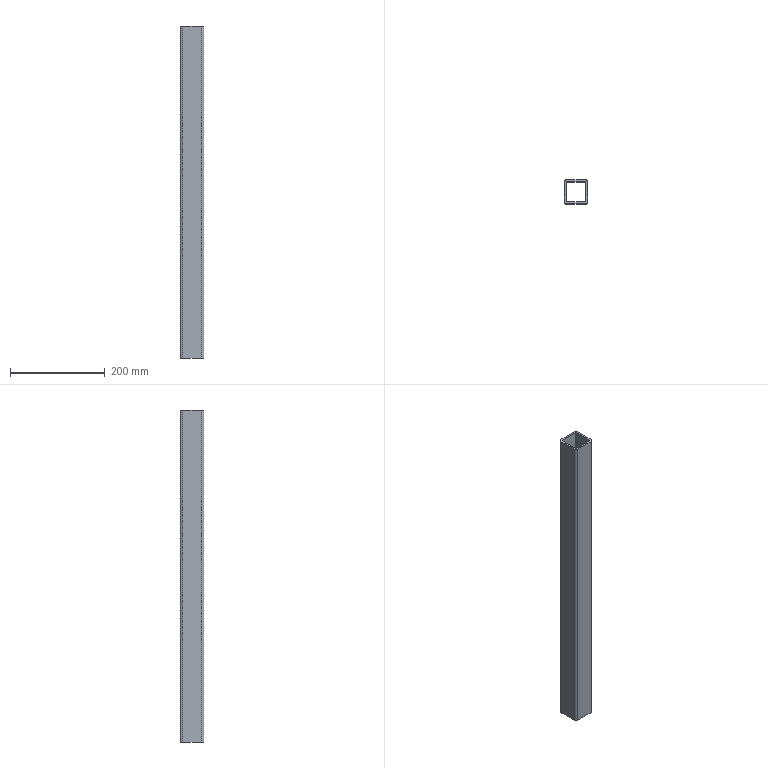Part | STEP file | Square steel 50×50×700 | 1 solid | 18 faces | box 50 x 50 x 700 mm | volume 500779 mm3 | plane 10 | cylinder 8 | commonest cylinder face diameters 2 x4 10 x4
STEP:
#1=CARTESIAN_POINT('',(0.,0.,0.));
#2=DIRECTION('',(0.,0.,1.));
#3=DIRECTION('',(1.,0.,0.));
#4=AXIS2_PLACEMENT_3D('',#1,#2,#3);
#5=CARTESIAN_POINT('',(-25.,-20.,350.));
#6=VERTEX_POINT('',#5);
#7=CARTESIAN_POINT('',(-20.,-25.,350.));
#8=VERTEX_POINT('',#7);
#9=CARTESIAN_POINT('',(-20.,-20.,350.));
#10=DIRECTION('',(0.,0.,1.));
#11=DIRECTION('',(1.,0.,0.));
#12=AXIS2_PLACEMENT_3D('',#9,#10,#11);
#13=CIRCLE('',#12,5.);
#14=CARTESIAN_POINT('',(-20.,-20.,350.));
#15=DIRECTION('',(0.,0.,1.));
#16=DIRECTION('',(1.,0.,0.));
#17=AXIS2_PLACEMENT_3D('',#14,#15,#16);
#18=PLANE('',#17);
#19=CARTESIAN_POINT('',(0.,0.));
#20=DIRECTION('',(1.,0.));
#21=AXIS2_PLACEMENT_2D('',#19,#20);
#22=CIRCLE('',#21,5.);
#23=(GEOMETRIC_REPRESENTATION_CONTEXT(2)PARAMETRIC_REPRESENTATION_CONTEXT()REPRESENTATION_CONTEXT('',''));
#24=DEFINITIONAL_REPRESENTATION('',(#22),#23);
#25=PCURVE('',#18,#24);
#26=CARTESIAN_POINT('',(-20.,-20.,350.));
#27=DIRECTION('',(0.,0.,-1.));
#28=DIRECTION('',(-1.,0.,0.));
#29=AXIS2_PLACEMENT_3D('',#26,#27,#28);
#30=CYLINDRICAL_SURFACE('',#29,5.);
#31=CARTESIAN_POINT('',(9.425,0.));
#32=DIRECTION('',(-1.,0.));
#33=VECTOR('',#32,1.);
#34=LINE('',#31,#33);
#35=(GEOMETRIC_REPRESENTATION_CONTEXT(2)PARAMETRIC_REPRESENTATION_CONTEXT()REPRESENTATION_CONTEXT('',''));
#36=DEFINITIONAL_REPRESENTATION('',(#34),#35);
#37=PCURVE('',#30,#36);
#38=SURFACE_CURVE('',#13,(#25,#37),.PCURVE_S1.);
#39=EDGE_CURVE('',#6,#8,#38,.T.);
#40=ORIENTED_EDGE('',*,*,#39,.T.);
#41=CARTESIAN_POINT('',(20.,-25.,350.));
#42=VERTEX_POINT('',#41);
#43=CARTESIAN_POINT('',(-20.,-25.,350.));
#44=DIRECTION('',(1.,0.,0.));
#45=VECTOR('',#44,1.);
#46=LINE('',#43,#45);
#47=CARTESIAN_POINT('',(0.,-5.));
#48=DIRECTION('',(1.,0.));
#49=VECTOR('',#48,1.);
#50=LINE('',#47,#49);
#51=(GEOMETRIC_REPRESENTATION_CONTEXT(2)PARAMETRIC_REPRESENTATION_CONTEXT()REPRESENTATION_CONTEXT('',''));
#52=DEFINITIONAL_REPRESENTATION('',(#50),#51);
#53=PCURVE('',#18,#52);
#54=CARTESIAN_POINT('',(-20.,-25.,350.));
#55=DIRECTION('',(0.,1.,0.));
#56=DIRECTION('',(0.,0.,1.));
#57=AXIS2_PLACEMENT_3D('',#54,#55,#56);
#58=PLANE('',#57);
#59=CARTESIAN_POINT('',(0.,0.));
#60=DIRECTION('',(0.,1.));
#61=VECTOR('',#60,1.);
#62=LINE('',#59,#61);
#63=(GEOMETRIC_REPRESENTATION_CONTEXT(2)PARAMETRIC_REPRESENTATION_CONTEXT()REPRESENTATION_CONTEXT('',''));
#64=DEFINITIONAL_REPRESENTATION('',(#62),#63);
#65=PCURVE('',#58,#64);
#66=SURFACE_CURVE('',#46,(#53,#65),.PCURVE_S1.);
#67=EDGE_CURVE('',#8,#42,#66,.T.);
#68=ORIENTED_EDGE('',*,*,#67,.T.);
#69=CARTESIAN_POINT('',(25.,-20.,350.));
#70=VERTEX_POINT('',#69);
#71=CARTESIAN_POINT('',(20.,-20.,350.));
#72=DIRECTION('',(0.,0.,1.));
#73=DIRECTION('',(-1.,0.,0.));
#74=AXIS2_PLACEMENT_3D('',#71,#72,#73);
#75=CIRCLE('',#74,5.);
#76=CARTESIAN_POINT('',(40.,0.));
#77=DIRECTION('',(-1.,0.));
#78=AXIS2_PLACEMENT_2D('',#76,#77);
#79=CIRCLE('',#78,5.);
#80=(GEOMETRIC_REPRESENTATION_CONTEXT(2)PARAMETRIC_REPRESENTATION_CONTEXT()REPRESENTATION_CONTEXT('',''));
#81=DEFINITIONAL_REPRESENTATION('',(#79),#80);
#82=PCURVE('',#18,#81);
#83=CARTESIAN_POINT('',(20.,-20.,350.));
#84=DIRECTION('',(0.,0.,-1.));
#85=DIRECTION('',(-1.,0.,0.));
#86=AXIS2_PLACEMENT_3D('',#83,#84,#85);
#87=CYLINDRICAL_SURFACE('',#86,5.);
#88=CARTESIAN_POINT('',(6.283,0.));
#89=DIRECTION('',(-1.,0.));
#90=VECTOR('',#89,1.);
#91=LINE('',#88,#90);
#92=(GEOMETRIC_REPRESENTATION_CONTEXT(2)PARAMETRIC_REPRESENTATION_CONTEXT()REPRESENTATION_CONTEXT('',''));
#93=DEFINITIONAL_REPRESENTATION('',(#91),#92);
#94=PCURVE('',#87,#93);
#95=SURFACE_CURVE('',#75,(#82,#94),.PCURVE_S1.);
#96=EDGE_CURVE('',#42,#70,#95,.T.);
#97=ORIENTED_EDGE('',*,*,#96,.T.);
#98=CARTESIAN_POINT('',(25.,20.,350.));
#99=VERTEX_POINT('',#98);
#100=CARTESIAN_POINT('',(25.,20.,350.));
#101=DIRECTION('',(0.,1.,0.));
#102=VECTOR('',#101,1.);
#103=LINE('',#100,#102);
#104=CARTESIAN_POINT('',(45.,40.));
#105=DIRECTION('',(0.,1.));
#106=VECTOR('',#105,1.);
#107=LINE('',#104,#106);
#108=(GEOMETRIC_REPRESENTATION_CONTEXT(2)PARAMETRIC_REPRESENTATION_CONTEXT()REPRESENTATION_CONTEXT('',''));
#109=DEFINITIONAL_REPRESENTATION('',(#107),#108);
#110=PCURVE('',#18,#109);
#111=CARTESIAN_POINT('',(25.,20.,350.));
#112=DIRECTION('',(-1.,0.,0.));
#113=DIRECTION('',(0.,-1.,0.));
#114=AXIS2_PLACEMENT_3D('',#111,#112,#113);
#115=PLANE('',#114);
#116=CARTESIAN_POINT('',(0.,0.));
#117=DIRECTION('',(-1.,0.));
#118=VECTOR('',#117,1.);
#119=LINE('',#116,#118);
#120=(GEOMETRIC_REPRESENTATION_CONTEXT(2)PARAMETRIC_REPRESENTATION_CONTEXT()REPRESENTATION_CONTEXT('',''));
#121=DEFINITIONAL_REPRESENTATION('',(#119),#120);
#122=PCURVE('',#115,#121);
#123=SURFACE_CURVE('',#103,(#110,#122),.PCURVE_S1.);
#124=EDGE_CURVE('',#70,#99,#123,.T.);
#125=ORIENTED_EDGE('',*,*,#124,.T.);
#126=CARTESIAN_POINT('',(20.,25.,350.));
#127=VERTEX_POINT('',#126);
#128=CARTESIAN_POINT('',(20.,20.,350.));
#129=DIRECTION('',(0.,0.,1.));
#130=DIRECTION('',(1.,0.,0.));
#131=AXIS2_PLACEMENT_3D('',#128,#129,#130);
#132=CIRCLE('',#131,5.);
#133=CARTESIAN_POINT('',(40.,40.));
#134=DIRECTION('',(1.,0.));
#135=AXIS2_PLACEMENT_2D('',#133,#134);
#136=CIRCLE('',#135,5.);
#137=(GEOMETRIC_REPRESENTATION_CONTEXT(2)PARAMETRIC_REPRESENTATION_CONTEXT()REPRESENTATION_CONTEXT('',''));
#138=DEFINITIONAL_REPRESENTATION('',(#136),#137);
#139=PCURVE('',#18,#138);
#140=CARTESIAN_POINT('',(20.,20.,350.));
#141=DIRECTION('',(0.,0.,-1.));
#142=DIRECTION('',(-1.,0.,0.));
#143=AXIS2_PLACEMENT_3D('',#140,#141,#142);
#144=CYLINDRICAL_SURFACE('',#143,5.);
#145=CARTESIAN_POINT('',(3.142,0.));
#146=DIRECTION('',(-1.,0.));
#147=VECTOR('',#146,1.);
#148=LINE('',#145,#147);
#149=(GEOMETRIC_REPRESENTATION_CONTEXT(2)PARAMETRIC_REPRESENTATION_CONTEXT()REPRESENTATION_CONTEXT('',''));
#150=DEFINITIONAL_REPRESENTATION('',(#148),#149);
#151=PCURVE('',#144,#150);
#152=SURFACE_CURVE('',#132,(#139,#151),.PCURVE_S1.);
#153=EDGE_CURVE('',#99,#127,#152,.T.);
#154=ORIENTED_EDGE('',*,*,#153,.T.);
#155=CARTESIAN_POINT('',(-20.,25.,350.));
#156=VERTEX_POINT('',#155);
#157=CARTESIAN_POINT('',(-20.,25.,350.));
#158=DIRECTION('',(-1.,0.,0.));
#159=VECTOR('',#158,1.);
#160=LINE('',#157,#159);
#161=CARTESIAN_POINT('',(0.,45.));
#162=DIRECTION('',(-1.,0.));
#163=VECTOR('',#162,1.);
#164=LINE('',#161,#163);
#165=(GEOMETRIC_REPRESENTATION_CONTEXT(2)PARAMETRIC_REPRESENTATION_CONTEXT()REPRESENTATION_CONTEXT('',''));
#166=DEFINITIONAL_REPRESENTATION('',(#164),#165);
#167=PCURVE('',#18,#166);
#168=CARTESIAN_POINT('',(-20.,25.,350.));
#169=DIRECTION('',(0.,-1.,0.));
#170=DIRECTION('',(0.,0.,-1.));
#171=AXIS2_PLACEMENT_3D('',#168,#169,#170);
#172=PLANE('',#171);
#173=CARTESIAN_POINT('',(0.,0.));
#174=DIRECTION('',(0.,-1.));
#175=VECTOR('',#174,1.);
#176=LINE('',#173,#175);
#177=(GEOMETRIC_REPRESENTATION_CONTEXT(2)PARAMETRIC_REPRESENTATION_CONTEXT()REPRESENTATION_CONTEXT('',''));
#178=DEFINITIONAL_REPRESENTATION('',(#176),#177);
#179=PCURVE('',#172,#178);
#180=SURFACE_CURVE('',#160,(#167,#179),.PCURVE_S1.);
#181=EDGE_CURVE('',#127,#156,#180,.T.);
#182=ORIENTED_EDGE('',*,*,#181,.T.);
#183=CARTESIAN_POINT('',(-25.,20.,350.));
#184=VERTEX_POINT('',#183);
#185=CARTESIAN_POINT('',(-20.,20.,350.));
#186=DIRECTION('',(0.,0.,1.));
#187=DIRECTION('',(-1.,0.,0.));
#188=AXIS2_PLACEMENT_3D('',#185,#186,#187);
#189=CIRCLE('',#188,5.);
#190=CARTESIAN_POINT('',(0.,40.));
#191=DIRECTION('',(-1.,0.));
#192=AXIS2_PLACEMENT_2D('',#190,#191);
#193=CIRCLE('',#192,5.);
#194=(GEOMETRIC_REPRESENTATION_CONTEXT(2)PARAMETRIC_REPRESENTATION_CONTEXT()REPRESENTATION_CONTEXT('',''));
#195=DEFINITIONAL_REPRESENTATION('',(#193),#194);
#196=PCURVE('',#18,#195);
#197=CARTESIAN_POINT('',(-20.,20.,350.));
#198=DIRECTION('',(0.,0.,-1.));
#199=DIRECTION('',(-1.,0.,0.));
#200=AXIS2_PLACEMENT_3D('',#197,#198,#199);
#201=CYLINDRICAL_SURFACE('',#200,5.);
#202=CARTESIAN_POINT('',(6.283,0.));
#203=DIRECTION('',(-1.,0.));
#204=VECTOR('',#203,1.);
#205=LINE('',#202,#204);
#206=(GEOMETRIC_REPRESENTATION_CONTEXT(2)PARAMETRIC_REPRESENTATION_CONTEXT()REPRESENTATION_CONTEXT('',''));
#207=DEFINITIONAL_REPRESENTATION('',(#205),#206);
#208=PCURVE('',#201,#207);
#209=SURFACE_CURVE('',#189,(#196,#208),.PCURVE_S1.);
#210=EDGE_CURVE('',#156,#184,#209,.T.);
#211=ORIENTED_EDGE('',*,*,#210,.T.);
#212=CARTESIAN_POINT('',(-25.,20.,350.));
#213=DIRECTION('',(0.,-1.,0.));
#214=VECTOR('',#213,1.);
#215=LINE('',#212,#214);
#216=CARTESIAN_POINT('',(-5.,40.));
#217=DIRECTION('',(0.,-1.));
#218=VECTOR('',#217,1.);
#219=LINE('',#216,#218);
#220=(GEOMETRIC_REPRESENTATION_CONTEXT(2)PARAMETRIC_REPRESENTATION_CONTEXT()REPRESENTATION_CONTEXT('',''));
#221=DEFINITIONAL_REPRESENTATION('',(#219),#220);
#222=PCURVE('',#18,#221);
#223=CARTESIAN_POINT('',(-25.,20.,350.));
#224=DIRECTION('',(1.,0.,0.));
#225=DIRECTION('',(0.,1.,0.));
#226=AXIS2_PLACEMENT_3D('',#223,#224,#225);
#227=PLANE('',#226);
#228=CARTESIAN_POINT('',(0.,0.));
#229=DIRECTION('',(-1.,0.));
#230=VECTOR('',#229,1.);
#231=LINE('',#228,#230);
#232=(GEOMETRIC_REPRESENTATION_CONTEXT(2)PARAMETRIC_REPRESENTATION_CONTEXT()REPRESENTATION_CONTEXT('',''));
#233=DEFINITIONAL_REPRESENTATION('',(#231),#232);
#234=PCURVE('',#227,#233);
#235=SURFACE_CURVE('',#215,(#222,#234),.PCURVE_S1.);
#236=EDGE_CURVE('',#184,#6,#235,.T.);
#237=ORIENTED_EDGE('',*,*,#236,.T.);
#238=EDGE_LOOP('',(#40,#68,#97,#125,#154,#182,#211,#237));
#239=FACE_BOUND('',#238,.T.);
#240=CARTESIAN_POINT('',(-21.,20.,350.));
#241=VERTEX_POINT('',#240);
#242=CARTESIAN_POINT('',(-21.,-20.,350.));
#243=VERTEX_POINT('',#242);
#244=CARTESIAN_POINT('',(-21.,20.,350.));
#245=DIRECTION('',(0.,-1.,0.));
#246=VECTOR('',#245,1.);
#247=LINE('',#244,#246);
#248=CARTESIAN_POINT('',(-1.,40.));
#249=DIRECTION('',(0.,-1.));
#250=VECTOR('',#249,1.);
#251=LINE('',#248,#250);
#252=(GEOMETRIC_REPRESENTATION_CONTEXT(2)PARAMETRIC_REPRESENTATION_CONTEXT()REPRESENTATION_CONTEXT('',''));
#253=DEFINITIONAL_REPRESENTATION('',(#251),#252);
#254=PCURVE('',#18,#253);
#255=CARTESIAN_POINT('',(-21.,20.,350.));
#256=DIRECTION('',(1.,0.,0.));
#257=DIRECTION('',(0.,1.,0.));
#258=AXIS2_PLACEMENT_3D('',#255,#256,#257);
#259=PLANE('',#258);
#260=CARTESIAN_POINT('',(0.,0.));
#261=DIRECTION('',(-1.,0.));
#262=VECTOR('',#261,1.);
#263=LINE('',#260,#262);
#264=(GEOMETRIC_REPRESENTATION_CONTEXT(2)PARAMETRIC_REPRESENTATION_CONTEXT()REPRESENTATION_CONTEXT('',''));
#265=DEFINITIONAL_REPRESENTATION('',(#263),#264);
#266=PCURVE('',#259,#265);
#267=SURFACE_CURVE('',#247,(#254,#266),.PCURVE_S1.);
#268=EDGE_CURVE('',#241,#243,#267,.T.);
#269=ORIENTED_EDGE('',*,*,#268,.F.);
#270=CARTESIAN_POINT('',(-20.,21.,350.));
#271=VERTEX_POINT('',#270);
#272=CARTESIAN_POINT('',(-20.,20.,350.));
#273=DIRECTION('',(0.,0.,1.));
#274=DIRECTION('',(-1.,0.,0.));
#275=AXIS2_PLACEMENT_3D('',#272,#273,#274);
#276=CIRCLE('',#275,1.);
#277=CARTESIAN_POINT('',(0.,40.));
#278=DIRECTION('',(-1.,0.));
#279=AXIS2_PLACEMENT_2D('',#277,#278);
#280=CIRCLE('',#279,1.);
#281=(GEOMETRIC_REPRESENTATION_CONTEXT(2)PARAMETRIC_REPRESENTATION_CONTEXT()REPRESENTATION_CONTEXT('',''));
#282=DEFINITIONAL_REPRESENTATION('',(#280),#281);
#283=PCURVE('',#18,#282);
#284=CARTESIAN_POINT('',(-20.,20.,350.));
#285=DIRECTION('',(0.,0.,-1.));
#286=DIRECTION('',(-1.,0.,0.));
#287=AXIS2_PLACEMENT_3D('',#284,#285,#286);
#288=CYLINDRICAL_SURFACE('',#287,1.);
#289=CARTESIAN_POINT('',(6.283,0.));
#290=DIRECTION('',(-1.,0.));
#291=VECTOR('',#290,1.);
#292=LINE('',#289,#291);
#293=(GEOMETRIC_REPRESENTATION_CONTEXT(2)PARAMETRIC_REPRESENTATION_CONTEXT()REPRESENTATION_CONTEXT('',''));
#294=DEFINITIONAL_REPRESENTATION('',(#292),#293);
#295=PCURVE('',#288,#294);
#296=SURFACE_CURVE('',#276,(#283,#295),.PCURVE_S1.);
#297=EDGE_CURVE('',#271,#241,#296,.T.);
#298=ORIENTED_EDGE('',*,*,#297,.F.);
#299=CARTESIAN_POINT('',(20.,21.,350.));
#300=VERTEX_POINT('',#299);
#301=CARTESIAN_POINT('',(-20.,21.,350.));
#302=DIRECTION('',(-1.,0.,0.));
#303=VECTOR('',#302,1.);
#304=LINE('',#301,#303);
#305=CARTESIAN_POINT('',(0.,41.));
#306=DIRECTION('',(-1.,0.));
#307=VECTOR('',#306,1.);
#308=LINE('',#305,#307);
#309=(GEOMETRIC_REPRESENTATION_CONTEXT(2)PARAMETRIC_REPRESENTATION_CONTEXT()REPRESENTATION_CONTEXT('',''));
#310=DEFINITIONAL_REPRESENTATION('',(#308),#309);
#311=PCURVE('',#18,#310);
#312=CARTESIAN_POINT('',(-20.,21.,350.));
#313=DIRECTION('',(0.,-1.,0.));
#314=DIRECTION('',(0.,0.,-1.));
#315=AXIS2_PLACEMENT_3D('',#312,#313,#314);
#316=PLANE('',#315);
#317=CARTESIAN_POINT('',(0.,0.));
#318=DIRECTION('',(0.,-1.));
#319=VECTOR('',#318,1.);
#320=LINE('',#317,#319);
#321=(GEOMETRIC_REPRESENTATION_CONTEXT(2)PARAMETRIC_REPRESENTATION_CONTEXT()REPRESENTATION_CONTEXT('',''));
#322=DEFINITIONAL_REPRESENTATION('',(#320),#321);
#323=PCURVE('',#316,#322);
#324=SURFACE_CURVE('',#304,(#311,#323),.PCURVE_S1.);
#325=EDGE_CURVE('',#300,#271,#324,.T.);
#326=ORIENTED_EDGE('',*,*,#325,.F.);
#327=CARTESIAN_POINT('',(21.,20.,350.));
#328=VERTEX_POINT('',#327);
#329=CARTESIAN_POINT('',(20.,20.,350.));
#330=DIRECTION('',(0.,0.,1.));
#331=DIRECTION('',(1.,0.,0.));
#332=AXIS2_PLACEMENT_3D('',#329,#330,#331);
#333=CIRCLE('',#332,1.);
#334=CARTESIAN_POINT('',(40.,40.));
#335=DIRECTION('',(1.,0.));
#336=AXIS2_PLACEMENT_2D('',#334,#335);
#337=CIRCLE('',#336,1.);
#338=(GEOMETRIC_REPRESENTATION_CONTEXT(2)PARAMETRIC_REPRESENTATION_CONTEXT()REPRESENTATION_CONTEXT('',''));
#339=DEFINITIONAL_REPRESENTATION('',(#337),#338);
#340=PCURVE('',#18,#339);
#341=CARTESIAN_POINT('',(20.,20.,350.));
#342=DIRECTION('',(0.,0.,-1.));
#343=DIRECTION('',(-1.,0.,0.));
#344=AXIS2_PLACEMENT_3D('',#341,#342,#343);
#345=CYLINDRICAL_SURFACE('',#344,1.);
#346=CARTESIAN_POINT('',(3.142,0.));
#347=DIRECTION('',(-1.,0.));
#348=VECTOR('',#347,1.);
#349=LINE('',#346,#348);
#350=(GEOMETRIC_REPRESENTATION_CONTEXT(2)PARAMETRIC_REPRESENTATION_CONTEXT()REPRESENTATION_CONTEXT('',''));
#351=DEFINITIONAL_REPRESENTATION('',(#349),#350);
#352=PCURVE('',#345,#351);
#353=SURFACE_CURVE('',#333,(#340,#352),.PCURVE_S1.);
#354=EDGE_CURVE('',#328,#300,#353,.T.);
#355=ORIENTED_EDGE('',*,*,#354,.F.);
#356=CARTESIAN_POINT('',(21.,-20.,350.));
#357=VERTEX_POINT('',#356);
#358=CARTESIAN_POINT('',(21.,20.,350.));
#359=DIRECTION('',(0.,1.,0.));
#360=VECTOR('',#359,1.);
#361=LINE('',#358,#360);
#362=CARTESIAN_POINT('',(41.,40.));
#363=DIRECTION('',(0.,1.));
#364=VECTOR('',#363,1.);
#365=LINE('',#362,#364);
#366=(GEOMETRIC_REPRESENTATION_CONTEXT(2)PARAMETRIC_REPRESENTATION_CONTEXT()REPRESENTATION_CONTEXT('',''));
#367=DEFINITIONAL_REPRESENTATION('',(#365),#366);
#368=PCURVE('',#18,#367);
#369=CARTESIAN_POINT('',(21.,20.,350.));
#370=DIRECTION('',(-1.,0.,0.));
#371=DIRECTION('',(0.,0.,1.));
#372=AXIS2_PLACEMENT_3D('',#369,#370,#371);
#373=PLANE('',#372);
#374=CARTESIAN_POINT('',(0.,0.));
#375=DIRECTION('',(0.,1.));
#376=VECTOR('',#375,1.);
#377=LINE('',#374,#376);
#378=(GEOMETRIC_REPRESENTATION_CONTEXT(2)PARAMETRIC_REPRESENTATION_CONTEXT()REPRESENTATION_CONTEXT('',''));
#379=DEFINITIONAL_REPRESENTATION('',(#377),#378);
#380=PCURVE('',#373,#379);
#381=SURFACE_CURVE('',#361,(#368,#380),.PCURVE_S1.);
#382=EDGE_CURVE('',#357,#328,#381,.T.);
#383=ORIENTED_EDGE('',*,*,#382,.F.);
#384=CARTESIAN_POINT('',(20.,-21.,350.));
#385=VERTEX_POINT('',#384);
#386=CARTESIAN_POINT('',(20.,-20.,350.));
#387=DIRECTION('',(0.,0.,1.));
#388=DIRECTION('',(-1.,0.,0.));
#389=AXIS2_PLACEMENT_3D('',#386,#387,#388);
#390=CIRCLE('',#389,1.);
#391=CARTESIAN_POINT('',(40.,0.));
#392=DIRECTION('',(-1.,0.));
#393=AXIS2_PLACEMENT_2D('',#391,#392);
#394=CIRCLE('',#393,1.);
#395=(GEOMETRIC_REPRESENTATION_CONTEXT(2)PARAMETRIC_REPRESENTATION_CONTEXT()REPRESENTATION_CONTEXT('',''));
#396=DEFINITIONAL_REPRESENTATION('',(#394),#395);
#397=PCURVE('',#18,#396);
#398=CARTESIAN_POINT('',(20.,-20.,350.));
#399=DIRECTION('',(0.,0.,-1.));
#400=DIRECTION('',(-1.,0.,0.));
#401=AXIS2_PLACEMENT_3D('',#398,#399,#400);
#402=CYLINDRICAL_SURFACE('',#401,1.);
#403=CARTESIAN_POINT('',(6.283,0.));
#404=DIRECTION('',(-1.,0.));
#405=VECTOR('',#404,1.);
#406=LINE('',#403,#405);
#407=(GEOMETRIC_REPRESENTATION_CONTEXT(2)PARAMETRIC_REPRESENTATION_CONTEXT()REPRESENTATION_CONTEXT('',''));
#408=DEFINITIONAL_REPRESENTATION('',(#406),#407);
#409=PCURVE('',#402,#408);
#410=SURFACE_CURVE('',#390,(#397,#409),.PCURVE_S1.);
#411=EDGE_CURVE('',#385,#357,#410,.T.);
#412=ORIENTED_EDGE('',*,*,#411,.F.);
#413=CARTESIAN_POINT('',(-20.,-21.,350.));
#414=VERTEX_POINT('',#413);
#415=CARTESIAN_POINT('',(-20.,-21.,350.));
#416=DIRECTION('',(1.,0.,0.));
#417=VECTOR('',#416,1.);
#418=LINE('',#415,#417);
#419=CARTESIAN_POINT('',(0.,-1.));
#420=DIRECTION('',(1.,0.));
#421=VECTOR('',#420,1.);
#422=LINE('',#419,#421);
#423=(GEOMETRIC_REPRESENTATION_CONTEXT(2)PARAMETRIC_REPRESENTATION_CONTEXT()REPRESENTATION_CONTEXT('',''));
#424=DEFINITIONAL_REPRESENTATION('',(#422),#423);
#425=PCURVE('',#18,#424);
#426=CARTESIAN_POINT('',(-20.,-21.,350.));
#427=DIRECTION('',(0.,1.,0.));
#428=DIRECTION('',(0.,0.,1.));
#429=AXIS2_PLACEMENT_3D('',#426,#427,#428);
#430=PLANE('',#429);
#431=CARTESIAN_POINT('',(0.,0.));
#432=DIRECTION('',(0.,1.));
#433=VECTOR('',#432,1.);
#434=LINE('',#431,#433);
#435=(GEOMETRIC_REPRESENTATION_CONTEXT(2)PARAMETRIC_REPRESENTATION_CONTEXT()REPRESENTATION_CONTEXT('',''));
#436=DEFINITIONAL_REPRESENTATION('',(#434),#435);
#437=PCURVE('',#430,#436);
#438=SURFACE_CURVE('',#418,(#425,#437),.PCURVE_S1.);
#439=EDGE_CURVE('',#414,#385,#438,.T.);
#440=ORIENTED_EDGE('',*,*,#439,.F.);
#441=CARTESIAN_POINT('',(-20.,-20.,350.));
#442=DIRECTION('',(0.,0.,1.));
#443=DIRECTION('',(1.,0.,0.));
#444=AXIS2_PLACEMENT_3D('',#441,#442,#443);
#445=CIRCLE('',#444,1.);
#446=CARTESIAN_POINT('',(0.,0.));
#447=DIRECTION('',(1.,0.));
#448=AXIS2_PLACEMENT_2D('',#446,#447);
#449=CIRCLE('',#448,1.);
#450=(GEOMETRIC_REPRESENTATION_CONTEXT(2)PARAMETRIC_REPRESENTATION_CONTEXT()REPRESENTATION_CONTEXT('',''));
#451=DEFINITIONAL_REPRESENTATION('',(#449),#450);
#452=PCURVE('',#18,#451);
#453=CARTESIAN_POINT('',(-20.,-20.,350.));
#454=DIRECTION('',(0.,0.,-1.));
#455=DIRECTION('',(-1.,0.,0.));
#456=AXIS2_PLACEMENT_3D('',#453,#454,#455);
#457=CYLINDRICAL_SURFACE('',#456,1.);
#458=CARTESIAN_POINT('',(9.425,0.));
#459=DIRECTION('',(-1.,0.));
#460=VECTOR('',#459,1.);
#461=LINE('',#458,#460);
#462=(GEOMETRIC_REPRESENTATION_CONTEXT(2)PARAMETRIC_REPRESENTATION_CONTEXT()REPRESENTATION_CONTEXT('',''));
#463=DEFINITIONAL_REPRESENTATION('',(#461),#462);
#464=PCURVE('',#457,#463);
#465=SURFACE_CURVE('',#445,(#452,#464),.PCURVE_S1.);
#466=EDGE_CURVE('',#243,#414,#465,.T.);
#467=ORIENTED_EDGE('',*,*,#466,.F.);
#468=EDGE_LOOP('',(#269,#298,#326,#355,#383,#412,#440,#467));
#469=FACE_BOUND('',#468,.T.);
#470=ADVANCED_FACE('',(#239,#469),#18,.T.);
#471=CARTESIAN_POINT('',(-25.,-20.,-350.));
#472=VERTEX_POINT('',#471);
#473=CARTESIAN_POINT('',(-20.,-25.,-350.));
#474=VERTEX_POINT('',#473);
#475=CARTESIAN_POINT('',(-20.,-20.,-350.));
#476=DIRECTION('',(0.,0.,1.));
#477=DIRECTION('',(1.,0.,0.));
#478=AXIS2_PLACEMENT_3D('',#475,#476,#477);
#479=CIRCLE('',#478,5.);
#480=CARTESIAN_POINT('',(-20.,-20.,-350.));
#481=DIRECTION('',(0.,0.,1.));
#482=DIRECTION('',(1.,0.,0.));
#483=AXIS2_PLACEMENT_3D('',#480,#481,#482);
#484=PLANE('',#483);
#485=CARTESIAN_POINT('',(0.,0.));
#486=DIRECTION('',(1.,0.));
#487=AXIS2_PLACEMENT_2D('',#485,#486);
#488=CIRCLE('',#487,5.);
#489=(GEOMETRIC_REPRESENTATION_CONTEXT(2)PARAMETRIC_REPRESENTATION_CONTEXT()REPRESENTATION_CONTEXT('',''));
#490=DEFINITIONAL_REPRESENTATION('',(#488),#489);
#491=PCURVE('',#484,#490);
#492=CARTESIAN_POINT('',(9.425,700.));
#493=DIRECTION('',(-1.,0.));
#494=VECTOR('',#493,1.);
#495=LINE('',#492,#494);
#496=(GEOMETRIC_REPRESENTATION_CONTEXT(2)PARAMETRIC_REPRESENTATION_CONTEXT()REPRESENTATION_CONTEXT('',''));
#497=DEFINITIONAL_REPRESENTATION('',(#495),#496);
#498=PCURVE('',#30,#497);
#499=SURFACE_CURVE('',#479,(#491,#498),.PCURVE_S1.);
#500=EDGE_CURVE('',#472,#474,#499,.T.);
#501=ORIENTED_EDGE('',*,*,#500,.F.);
#502=CARTESIAN_POINT('',(-25.,20.,-350.));
#503=VERTEX_POINT('',#502);
#504=CARTESIAN_POINT('',(-25.,20.,-350.));
#505=DIRECTION('',(0.,-1.,0.));
#506=VECTOR('',#505,1.);
#507=LINE('',#504,#506);
#508=CARTESIAN_POINT('',(-5.,40.));
#509=DIRECTION('',(0.,-1.));
#510=VECTOR('',#509,1.);
#511=LINE('',#508,#510);
#512=(GEOMETRIC_REPRESENTATION_CONTEXT(2)PARAMETRIC_REPRESENTATION_CONTEXT()REPRESENTATION_CONTEXT('',''));
#513=DEFINITIONAL_REPRESENTATION('',(#511),#512);
#514=PCURVE('',#484,#513);
#515=CARTESIAN_POINT('',(0.,-700.));
#516=DIRECTION('',(-1.,0.));
#517=VECTOR('',#516,1.);
#518=LINE('',#515,#517);
#519=(GEOMETRIC_REPRESENTATION_CONTEXT(2)PARAMETRIC_REPRESENTATION_CONTEXT()REPRESENTATION_CONTEXT('',''));
#520=DEFINITIONAL_REPRESENTATION('',(#518),#519);
#521=PCURVE('',#227,#520);
#522=SURFACE_CURVE('',#507,(#514,#521),.PCURVE_S1.);
#523=EDGE_CURVE('',#503,#472,#522,.T.);
#524=ORIENTED_EDGE('',*,*,#523,.F.);
#525=CARTESIAN_POINT('',(-20.,25.,-350.));
#526=VERTEX_POINT('',#525);
#527=CARTESIAN_POINT('',(-20.,20.,-350.));
#528=DIRECTION('',(0.,0.,1.));
#529=DIRECTION('',(-1.,0.,0.));
#530=AXIS2_PLACEMENT_3D('',#527,#528,#529);
#531=CIRCLE('',#530,5.);
#532=CARTESIAN_POINT('',(0.,40.));
#533=DIRECTION('',(-1.,0.));
#534=AXIS2_PLACEMENT_2D('',#532,#533);
#535=CIRCLE('',#534,5.);
#536=(GEOMETRIC_REPRESENTATION_CONTEXT(2)PARAMETRIC_REPRESENTATION_CONTEXT()REPRESENTATION_CONTEXT('',''));
#537=DEFINITIONAL_REPRESENTATION('',(#535),#536);
#538=PCURVE('',#484,#537);
#539=CARTESIAN_POINT('',(6.283,700.));
#540=DIRECTION('',(-1.,0.));
#541=VECTOR('',#540,1.);
#542=LINE('',#539,#541);
#543=(GEOMETRIC_REPRESENTATION_CONTEXT(2)PARAMETRIC_REPRESENTATION_CONTEXT()REPRESENTATION_CONTEXT('',''));
#544=DEFINITIONAL_REPRESENTATION('',(#542),#543);
#545=PCURVE('',#201,#544);
#546=SURFACE_CURVE('',#531,(#538,#545),.PCURVE_S1.);
#547=EDGE_CURVE('',#526,#503,#546,.T.);
#548=ORIENTED_EDGE('',*,*,#547,.F.);
#549=CARTESIAN_POINT('',(20.,25.,-350.));
#550=VERTEX_POINT('',#549);
#551=CARTESIAN_POINT('',(-20.,25.,-350.));
#552=DIRECTION('',(-1.,0.,0.));
#553=VECTOR('',#552,1.);
#554=LINE('',#551,#553);
#555=CARTESIAN_POINT('',(0.,45.));
#556=DIRECTION('',(-1.,0.));
#557=VECTOR('',#556,1.);
#558=LINE('',#555,#557);
#559=(GEOMETRIC_REPRESENTATION_CONTEXT(2)PARAMETRIC_REPRESENTATION_CONTEXT()REPRESENTATION_CONTEXT('',''));
#560=DEFINITIONAL_REPRESENTATION('',(#558),#559);
#561=PCURVE('',#484,#560);
#562=CARTESIAN_POINT('',(700.,0.));
#563=DIRECTION('',(0.,-1.));
#564=VECTOR('',#563,1.);
#565=LINE('',#562,#564);
#566=(GEOMETRIC_REPRESENTATION_CONTEXT(2)PARAMETRIC_REPRESENTATION_CONTEXT()REPRESENTATION_CONTEXT('',''));
#567=DEFINITIONAL_REPRESENTATION('',(#565),#566);
#568=PCURVE('',#172,#567);
#569=SURFACE_CURVE('',#554,(#561,#568),.PCURVE_S1.);
#570=EDGE_CURVE('',#550,#526,#569,.T.);
#571=ORIENTED_EDGE('',*,*,#570,.F.);
#572=CARTESIAN_POINT('',(25.,20.,-350.));
#573=VERTEX_POINT('',#572);
#574=CARTESIAN_POINT('',(20.,20.,-350.));
#575=DIRECTION('',(0.,0.,1.));
#576=DIRECTION('',(1.,0.,0.));
#577=AXIS2_PLACEMENT_3D('',#574,#575,#576);
#578=CIRCLE('',#577,5.);
#579=CARTESIAN_POINT('',(40.,40.));
#580=DIRECTION('',(1.,0.));
#581=AXIS2_PLACEMENT_2D('',#579,#580);
#582=CIRCLE('',#581,5.);
#583=(GEOMETRIC_REPRESENTATION_CONTEXT(2)PARAMETRIC_REPRESENTATION_CONTEXT()REPRESENTATION_CONTEXT('',''));
#584=DEFINITIONAL_REPRESENTATION('',(#582),#583);
#585=PCURVE('',#484,#584);
#586=CARTESIAN_POINT('',(3.142,700.));
#587=DIRECTION('',(-1.,0.));
#588=VECTOR('',#587,1.);
#589=LINE('',#586,#588);
#590=(GEOMETRIC_REPRESENTATION_CONTEXT(2)PARAMETRIC_REPRESENTATION_CONTEXT()REPRESENTATION_CONTEXT('',''));
#591=DEFINITIONAL_REPRESENTATION('',(#589),#590);
#592=PCURVE('',#144,#591);
#593=SURFACE_CURVE('',#578,(#585,#592),.PCURVE_S1.);
#594=EDGE_CURVE('',#573,#550,#593,.T.);
#595=ORIENTED_EDGE('',*,*,#594,.F.);
#596=CARTESIAN_POINT('',(25.,-20.,-350.));
#597=VERTEX_POINT('',#596);
#598=CARTESIAN_POINT('',(25.,20.,-350.));
#599=DIRECTION('',(0.,1.,0.));
#600=VECTOR('',#599,1.);
#601=LINE('',#598,#600);
#602=CARTESIAN_POINT('',(45.,40.));
#603=DIRECTION('',(0.,1.));
#604=VECTOR('',#603,1.);
#605=LINE('',#602,#604);
#606=(GEOMETRIC_REPRESENTATION_CONTEXT(2)PARAMETRIC_REPRESENTATION_CONTEXT()REPRESENTATION_CONTEXT('',''));
#607=DEFINITIONAL_REPRESENTATION('',(#605),#606);
#608=PCURVE('',#484,#607);
#609=CARTESIAN_POINT('',(0.,-700.));
#610=DIRECTION('',(-1.,0.));
#611=VECTOR('',#610,1.);
#612=LINE('',#609,#611);
#613=(GEOMETRIC_REPRESENTATION_CONTEXT(2)PARAMETRIC_REPRESENTATION_CONTEXT()REPRESENTATION_CONTEXT('',''));
#614=DEFINITIONAL_REPRESENTATION('',(#612),#613);
#615=PCURVE('',#115,#614);
#616=SURFACE_CURVE('',#601,(#608,#615),.PCURVE_S1.);
#617=EDGE_CURVE('',#597,#573,#616,.T.);
#618=ORIENTED_EDGE('',*,*,#617,.F.);
#619=CARTESIAN_POINT('',(20.,-25.,-350.));
#620=VERTEX_POINT('',#619);
#621=CARTESIAN_POINT('',(20.,-20.,-350.));
#622=DIRECTION('',(0.,0.,1.));
#623=DIRECTION('',(-1.,0.,0.));
#624=AXIS2_PLACEMENT_3D('',#621,#622,#623);
#625=CIRCLE('',#624,5.);
#626=CARTESIAN_POINT('',(40.,0.));
#627=DIRECTION('',(-1.,0.));
#628=AXIS2_PLACEMENT_2D('',#626,#627);
#629=CIRCLE('',#628,5.);
#630=(GEOMETRIC_REPRESENTATION_CONTEXT(2)PARAMETRIC_REPRESENTATION_CONTEXT()REPRESENTATION_CONTEXT('',''));
#631=DEFINITIONAL_REPRESENTATION('',(#629),#630);
#632=PCURVE('',#484,#631);
#633=CARTESIAN_POINT('',(6.283,700.));
#634=DIRECTION('',(-1.,0.));
#635=VECTOR('',#634,1.);
#636=LINE('',#633,#635);
#637=(GEOMETRIC_REPRESENTATION_CONTEXT(2)PARAMETRIC_REPRESENTATION_CONTEXT()REPRESENTATION_CONTEXT('',''));
#638=DEFINITIONAL_REPRESENTATION('',(#636),#637);
#639=PCURVE('',#87,#638);
#640=SURFACE_CURVE('',#625,(#632,#639),.PCURVE_S1.);
#641=EDGE_CURVE('',#620,#597,#640,.T.);
#642=ORIENTED_EDGE('',*,*,#641,.F.);
#643=CARTESIAN_POINT('',(-20.,-25.,-350.));
#644=DIRECTION('',(1.,0.,0.));
#645=VECTOR('',#644,1.);
#646=LINE('',#643,#645);
#647=CARTESIAN_POINT('',(0.,-5.));
#648=DIRECTION('',(1.,0.));
#649=VECTOR('',#648,1.);
#650=LINE('',#647,#649);
#651=(GEOMETRIC_REPRESENTATION_CONTEXT(2)PARAMETRIC_REPRESENTATION_CONTEXT()REPRESENTATION_CONTEXT('',''));
#652=DEFINITIONAL_REPRESENTATION('',(#650),#651);
#653=PCURVE('',#484,#652);
#654=CARTESIAN_POINT('',(-700.,0.));
#655=DIRECTION('',(0.,1.));
#656=VECTOR('',#655,1.);
#657=LINE('',#654,#656);
#658=(GEOMETRIC_REPRESENTATION_CONTEXT(2)PARAMETRIC_REPRESENTATION_CONTEXT()REPRESENTATION_CONTEXT('',''));
#659=DEFINITIONAL_REPRESENTATION('',(#657),#658);
#660=PCURVE('',#58,#659);
#661=SURFACE_CURVE('',#646,(#653,#660),.PCURVE_S1.);
#662=EDGE_CURVE('',#474,#620,#661,.T.);
#663=ORIENTED_EDGE('',*,*,#662,.F.);
#664=EDGE_LOOP('',(#501,#524,#548,#571,#595,#618,#642,#663));
#665=FACE_BOUND('',#664,.T.);
#666=CARTESIAN_POINT('',(-20.,21.,-350.));
#667=VERTEX_POINT('',#666);
#668=CARTESIAN_POINT('',(-21.,20.,-350.));
#669=VERTEX_POINT('',#668);
#670=CARTESIAN_POINT('',(-20.,20.,-350.));
#671=DIRECTION('',(0.,0.,1.));
#672=DIRECTION('',(-1.,0.,0.));
#673=AXIS2_PLACEMENT_3D('',#670,#671,#672);
#674=CIRCLE('',#673,1.);
#675=CARTESIAN_POINT('',(0.,40.));
#676=DIRECTION('',(-1.,0.));
#677=AXIS2_PLACEMENT_2D('',#675,#676);
#678=CIRCLE('',#677,1.);
#679=(GEOMETRIC_REPRESENTATION_CONTEXT(2)PARAMETRIC_REPRESENTATION_CONTEXT()REPRESENTATION_CONTEXT('',''));
#680=DEFINITIONAL_REPRESENTATION('',(#678),#679);
#681=PCURVE('',#484,#680);
#682=CARTESIAN_POINT('',(6.283,700.));
#683=DIRECTION('',(-1.,0.));
#684=VECTOR('',#683,1.);
#685=LINE('',#682,#684);
#686=(GEOMETRIC_REPRESENTATION_CONTEXT(2)PARAMETRIC_REPRESENTATION_CONTEXT()REPRESENTATION_CONTEXT('',''));
#687=DEFINITIONAL_REPRESENTATION('',(#685),#686);
#688=PCURVE('',#288,#687);
#689=SURFACE_CURVE('',#674,(#681,#688),.PCURVE_S1.);
#690=EDGE_CURVE('',#667,#669,#689,.T.);
#691=ORIENTED_EDGE('',*,*,#690,.T.);
#692=CARTESIAN_POINT('',(-21.,-20.,-350.));
#693=VERTEX_POINT('',#692);
#694=CARTESIAN_POINT('',(-21.,20.,-350.));
#695=DIRECTION('',(0.,-1.,0.));
#696=VECTOR('',#695,1.);
#697=LINE('',#694,#696);
#698=CARTESIAN_POINT('',(-1.,40.));
#699=DIRECTION('',(0.,-1.));
#700=VECTOR('',#699,1.);
#701=LINE('',#698,#700);
#702=(GEOMETRIC_REPRESENTATION_CONTEXT(2)PARAMETRIC_REPRESENTATION_CONTEXT()REPRESENTATION_CONTEXT('',''));
#703=DEFINITIONAL_REPRESENTATION('',(#701),#702);
#704=PCURVE('',#484,#703);
#705=CARTESIAN_POINT('',(0.,-700.));
#706=DIRECTION('',(-1.,0.));
#707=VECTOR('',#706,1.);
#708=LINE('',#705,#707);
#709=(GEOMETRIC_REPRESENTATION_CONTEXT(2)PARAMETRIC_REPRESENTATION_CONTEXT()REPRESENTATION_CONTEXT('',''));
#710=DEFINITIONAL_REPRESENTATION('',(#708),#709);
#711=PCURVE('',#259,#710);
#712=SURFACE_CURVE('',#697,(#704,#711),.PCURVE_S1.);
#713=EDGE_CURVE('',#669,#693,#712,.T.);
#714=ORIENTED_EDGE('',*,*,#713,.T.);
#715=CARTESIAN_POINT('',(-20.,-21.,-350.));
#716=VERTEX_POINT('',#715);
#717=CARTESIAN_POINT('',(-20.,-20.,-350.));
#718=DIRECTION('',(0.,0.,1.));
#719=DIRECTION('',(1.,0.,0.));
#720=AXIS2_PLACEMENT_3D('',#717,#718,#719);
#721=CIRCLE('',#720,1.);
#722=CARTESIAN_POINT('',(0.,0.));
#723=DIRECTION('',(1.,0.));
#724=AXIS2_PLACEMENT_2D('',#722,#723);
#725=CIRCLE('',#724,1.);
#726=(GEOMETRIC_REPRESENTATION_CONTEXT(2)PARAMETRIC_REPRESENTATION_CONTEXT()REPRESENTATION_CONTEXT('',''));
#727=DEFINITIONAL_REPRESENTATION('',(#725),#726);
#728=PCURVE('',#484,#727);
#729=CARTESIAN_POINT('',(9.425,700.));
#730=DIRECTION('',(-1.,0.));
#731=VECTOR('',#730,1.);
#732=LINE('',#729,#731);
#733=(GEOMETRIC_REPRESENTATION_CONTEXT(2)PARAMETRIC_REPRESENTATION_CONTEXT()REPRESENTATION_CONTEXT('',''));
#734=DEFINITIONAL_REPRESENTATION('',(#732),#733);
#735=PCURVE('',#457,#734);
#736=SURFACE_CURVE('',#721,(#728,#735),.PCURVE_S1.);
#737=EDGE_CURVE('',#693,#716,#736,.T.);
#738=ORIENTED_EDGE('',*,*,#737,.T.);
#739=CARTESIAN_POINT('',(20.,-21.,-350.));
#740=VERTEX_POINT('',#739);
#741=CARTESIAN_POINT('',(-20.,-21.,-350.));
#742=DIRECTION('',(1.,0.,0.));
#743=VECTOR('',#742,1.);
#744=LINE('',#741,#743);
#745=CARTESIAN_POINT('',(0.,-1.));
#746=DIRECTION('',(1.,0.));
#747=VECTOR('',#746,1.);
#748=LINE('',#745,#747);
#749=(GEOMETRIC_REPRESENTATION_CONTEXT(2)PARAMETRIC_REPRESENTATION_CONTEXT()REPRESENTATION_CONTEXT('',''));
#750=DEFINITIONAL_REPRESENTATION('',(#748),#749);
#751=PCURVE('',#484,#750);
#752=CARTESIAN_POINT('',(-700.,0.));
#753=DIRECTION('',(0.,1.));
#754=VECTOR('',#753,1.);
#755=LINE('',#752,#754);
#756=(GEOMETRIC_REPRESENTATION_CONTEXT(2)PARAMETRIC_REPRESENTATION_CONTEXT()REPRESENTATION_CONTEXT('',''));
#757=DEFINITIONAL_REPRESENTATION('',(#755),#756);
#758=PCURVE('',#430,#757);
#759=SURFACE_CURVE('',#744,(#751,#758),.PCURVE_S1.);
#760=EDGE_CURVE('',#716,#740,#759,.T.);
#761=ORIENTED_EDGE('',*,*,#760,.T.);
#762=CARTESIAN_POINT('',(21.,-20.,-350.));
#763=VERTEX_POINT('',#762);
#764=CARTESIAN_POINT('',(20.,-20.,-350.));
#765=DIRECTION('',(0.,0.,1.));
#766=DIRECTION('',(-1.,0.,0.));
#767=AXIS2_PLACEMENT_3D('',#764,#765,#766);
#768=CIRCLE('',#767,1.);
#769=CARTESIAN_POINT('',(40.,0.));
#770=DIRECTION('',(-1.,0.));
#771=AXIS2_PLACEMENT_2D('',#769,#770);
#772=CIRCLE('',#771,1.);
#773=(GEOMETRIC_REPRESENTATION_CONTEXT(2)PARAMETRIC_REPRESENTATION_CONTEXT()REPRESENTATION_CONTEXT('',''));
#774=DEFINITIONAL_REPRESENTATION('',(#772),#773);
#775=PCURVE('',#484,#774);
#776=CARTESIAN_POINT('',(6.283,700.));
#777=DIRECTION('',(-1.,0.));
#778=VECTOR('',#777,1.);
#779=LINE('',#776,#778);
#780=(GEOMETRIC_REPRESENTATION_CONTEXT(2)PARAMETRIC_REPRESENTATION_CONTEXT()REPRESENTATION_CONTEXT('',''));
#781=DEFINITIONAL_REPRESENTATION('',(#779),#780);
#782=PCURVE('',#402,#781);
#783=SURFACE_CURVE('',#768,(#775,#782),.PCURVE_S1.);
#784=EDGE_CURVE('',#740,#763,#783,.T.);
#785=ORIENTED_EDGE('',*,*,#784,.T.);
#786=CARTESIAN_POINT('',(21.,20.,-350.));
#787=VERTEX_POINT('',#786);
#788=CARTESIAN_POINT('',(21.,20.,-350.));
#789=DIRECTION('',(0.,1.,0.));
#790=VECTOR('',#789,1.);
#791=LINE('',#788,#790);
#792=CARTESIAN_POINT('',(41.,40.));
#793=DIRECTION('',(0.,1.));
#794=VECTOR('',#793,1.);
#795=LINE('',#792,#794);
#796=(GEOMETRIC_REPRESENTATION_CONTEXT(2)PARAMETRIC_REPRESENTATION_CONTEXT()REPRESENTATION_CONTEXT('',''));
#797=DEFINITIONAL_REPRESENTATION('',(#795),#796);
#798=PCURVE('',#484,#797);
#799=CARTESIAN_POINT('',(-700.,0.));
#800=DIRECTION('',(0.,1.));
#801=VECTOR('',#800,1.);
#802=LINE('',#799,#801);
#803=(GEOMETRIC_REPRESENTATION_CONTEXT(2)PARAMETRIC_REPRESENTATION_CONTEXT()REPRESENTATION_CONTEXT('',''));
#804=DEFINITIONAL_REPRESENTATION('',(#802),#803);
#805=PCURVE('',#373,#804);
#806=SURFACE_CURVE('',#791,(#798,#805),.PCURVE_S1.);
#807=EDGE_CURVE('',#763,#787,#806,.T.);
#808=ORIENTED_EDGE('',*,*,#807,.T.);
#809=CARTESIAN_POINT('',(20.,21.,-350.));
#810=VERTEX_POINT('',#809);
#811=CARTESIAN_POINT('',(20.,20.,-350.));
#812=DIRECTION('',(0.,0.,1.));
#813=DIRECTION('',(1.,0.,0.));
#814=AXIS2_PLACEMENT_3D('',#811,#812,#813);
#815=CIRCLE('',#814,1.);
#816=CARTESIAN_POINT('',(40.,40.));
#817=DIRECTION('',(1.,0.));
#818=AXIS2_PLACEMENT_2D('',#816,#817);
#819=CIRCLE('',#818,1.);
#820=(GEOMETRIC_REPRESENTATION_CONTEXT(2)PARAMETRIC_REPRESENTATION_CONTEXT()REPRESENTATION_CONTEXT('',''));
#821=DEFINITIONAL_REPRESENTATION('',(#819),#820);
#822=PCURVE('',#484,#821);
#823=CARTESIAN_POINT('',(3.142,700.));
#824=DIRECTION('',(-1.,0.));
#825=VECTOR('',#824,1.);
#826=LINE('',#823,#825);
#827=(GEOMETRIC_REPRESENTATION_CONTEXT(2)PARAMETRIC_REPRESENTATION_CONTEXT()REPRESENTATION_CONTEXT('',''));
#828=DEFINITIONAL_REPRESENTATION('',(#826),#827);
#829=PCURVE('',#345,#828);
#830=SURFACE_CURVE('',#815,(#822,#829),.PCURVE_S1.);
#831=EDGE_CURVE('',#787,#810,#830,.T.);
#832=ORIENTED_EDGE('',*,*,#831,.T.);
#833=CARTESIAN_POINT('',(-20.,21.,-350.));
#834=DIRECTION('',(-1.,0.,0.));
#835=VECTOR('',#834,1.);
#836=LINE('',#833,#835);
#837=CARTESIAN_POINT('',(0.,41.));
#838=DIRECTION('',(-1.,0.));
#839=VECTOR('',#838,1.);
#840=LINE('',#837,#839);
#841=(GEOMETRIC_REPRESENTATION_CONTEXT(2)PARAMETRIC_REPRESENTATION_CONTEXT()REPRESENTATION_CONTEXT('',''));
#842=DEFINITIONAL_REPRESENTATION('',(#840),#841);
#843=PCURVE('',#484,#842);
#844=CARTESIAN_POINT('',(700.,0.));
#845=DIRECTION('',(0.,-1.));
#846=VECTOR('',#845,1.);
#847=LINE('',#844,#846);
#848=(GEOMETRIC_REPRESENTATION_CONTEXT(2)PARAMETRIC_REPRESENTATION_CONTEXT()REPRESENTATION_CONTEXT('',''));
#849=DEFINITIONAL_REPRESENTATION('',(#847),#848);
#850=PCURVE('',#316,#849);
#851=SURFACE_CURVE('',#836,(#843,#850),.PCURVE_S1.);
#852=EDGE_CURVE('',#810,#667,#851,.T.);
#853=ORIENTED_EDGE('',*,*,#852,.T.);
#854=EDGE_LOOP('',(#691,#714,#738,#761,#785,#808,#832,#853));
#855=FACE_BOUND('',#854,.T.);
#856=ADVANCED_FACE('',(#665,#855),#484,.F.);
#857=ORIENTED_EDGE('',*,*,#500,.T.);
#858=CARTESIAN_POINT('',(-20.,-25.,350.));
#859=DIRECTION('',(0.,0.,-1.));
#860=VECTOR('',#859,1.);
#861=LINE('',#858,#860);
#862=CARTESIAN_POINT('',(4.712,0.));
#863=DIRECTION('',(0.,1.));
#864=VECTOR('',#863,1.);
#865=LINE('',#862,#864);
#866=(GEOMETRIC_REPRESENTATION_CONTEXT(2)PARAMETRIC_REPRESENTATION_CONTEXT()REPRESENTATION_CONTEXT('',''));
#867=DEFINITIONAL_REPRESENTATION('',(#865),#866);
#868=PCURVE('',#30,#867);
#869=CARTESIAN_POINT('',(0.,0.));
#870=DIRECTION('',(-1.,0.));
#871=VECTOR('',#870,1.);
#872=LINE('',#869,#871);
#873=(GEOMETRIC_REPRESENTATION_CONTEXT(2)PARAMETRIC_REPRESENTATION_CONTEXT()REPRESENTATION_CONTEXT('',''));
#874=DEFINITIONAL_REPRESENTATION('',(#872),#873);
#875=PCURVE('',#58,#874);
#876=SURFACE_CURVE('',#861,(#868,#875),.PCURVE_S1.);
#877=EDGE_CURVE('',#8,#474,#876,.T.);
#878=ORIENTED_EDGE('',*,*,#877,.F.);
#879=ORIENTED_EDGE('',*,*,#39,.F.);
#880=CARTESIAN_POINT('',(-25.,-20.,350.));
#881=DIRECTION('',(0.,0.,-1.));
#882=VECTOR('',#881,1.);
#883=LINE('',#880,#882);
#884=CARTESIAN_POINT('',(6.283,0.));
#885=DIRECTION('',(0.,1.));
#886=VECTOR('',#885,1.);
#887=LINE('',#884,#886);
#888=(GEOMETRIC_REPRESENTATION_CONTEXT(2)PARAMETRIC_REPRESENTATION_CONTEXT()REPRESENTATION_CONTEXT('',''));
#889=DEFINITIONAL_REPRESENTATION('',(#887),#888);
#890=PCURVE('',#30,#889);
#891=CARTESIAN_POINT('',(-40.,0.));
#892=DIRECTION('',(0.,-1.));
#893=VECTOR('',#892,1.);
#894=LINE('',#891,#893);
#895=(GEOMETRIC_REPRESENTATION_CONTEXT(2)PARAMETRIC_REPRESENTATION_CONTEXT()REPRESENTATION_CONTEXT('',''));
#896=DEFINITIONAL_REPRESENTATION('',(#894),#895);
#897=PCURVE('',#227,#896);
#898=SURFACE_CURVE('',#883,(#890,#897),.PCURVE_S1.);
#899=EDGE_CURVE('',#6,#472,#898,.T.);
#900=ORIENTED_EDGE('',*,*,#899,.T.);
#901=EDGE_LOOP('',(#857,#878,#879,#900));
#902=FACE_BOUND('',#901,.T.);
#903=ADVANCED_FACE('',(#902),#30,.T.);
#904=ORIENTED_EDGE('',*,*,#662,.T.);
#905=CARTESIAN_POINT('',(20.,-25.,350.));
#906=DIRECTION('',(0.,0.,-1.));
#907=VECTOR('',#906,1.);
#908=LINE('',#905,#907);
#909=CARTESIAN_POINT('',(0.,40.));
#910=DIRECTION('',(-1.,0.));
#911=VECTOR('',#910,1.);
#912=LINE('',#909,#911);
#913=(GEOMETRIC_REPRESENTATION_CONTEXT(2)PARAMETRIC_REPRESENTATION_CONTEXT()REPRESENTATION_CONTEXT('',''));
#914=DEFINITIONAL_REPRESENTATION('',(#912),#913);
#915=PCURVE('',#58,#914);
#916=CARTESIAN_POINT('',(4.712,0.));
#917=DIRECTION('',(0.,1.));
#918=VECTOR('',#917,1.);
#919=LINE('',#916,#918);
#920=(GEOMETRIC_REPRESENTATION_CONTEXT(2)PARAMETRIC_REPRESENTATION_CONTEXT()REPRESENTATION_CONTEXT('',''));
#921=DEFINITIONAL_REPRESENTATION('',(#919),#920);
#922=PCURVE('',#87,#921);
#923=SURFACE_CURVE('',#908,(#915,#922),.PCURVE_S1.);
#924=EDGE_CURVE('',#42,#620,#923,.T.);
#925=ORIENTED_EDGE('',*,*,#924,.F.);
#926=ORIENTED_EDGE('',*,*,#67,.F.);
#927=ORIENTED_EDGE('',*,*,#877,.T.);
#928=EDGE_LOOP('',(#904,#925,#926,#927));
#929=FACE_BOUND('',#928,.T.);
#930=ADVANCED_FACE('',(#929),#58,.F.);
#931=ORIENTED_EDGE('',*,*,#641,.T.);
#932=CARTESIAN_POINT('',(25.,-20.,350.));
#933=DIRECTION('',(0.,0.,-1.));
#934=VECTOR('',#933,1.);
#935=LINE('',#932,#934);
#936=CARTESIAN_POINT('',(3.142,0.));
#937=DIRECTION('',(0.,1.));
#938=VECTOR('',#937,1.);
#939=LINE('',#936,#938);
#940=(GEOMETRIC_REPRESENTATION_CONTEXT(2)PARAMETRIC_REPRESENTATION_CONTEXT()REPRESENTATION_CONTEXT('',''));
#941=DEFINITIONAL_REPRESENTATION('',(#939),#940);
#942=PCURVE('',#87,#941);
#943=CARTESIAN_POINT('',(40.,0.));
#944=DIRECTION('',(0.,-1.));
#945=VECTOR('',#944,1.);
#946=LINE('',#943,#945);
#947=(GEOMETRIC_REPRESENTATION_CONTEXT(2)PARAMETRIC_REPRESENTATION_CONTEXT()REPRESENTATION_CONTEXT('',''));
#948=DEFINITIONAL_REPRESENTATION('',(#946),#947);
#949=PCURVE('',#115,#948);
#950=SURFACE_CURVE('',#935,(#942,#949),.PCURVE_S1.);
#951=EDGE_CURVE('',#70,#597,#950,.T.);
#952=ORIENTED_EDGE('',*,*,#951,.F.);
#953=ORIENTED_EDGE('',*,*,#96,.F.);
#954=ORIENTED_EDGE('',*,*,#924,.T.);
#955=EDGE_LOOP('',(#931,#952,#953,#954));
#956=FACE_BOUND('',#955,.T.);
#957=ADVANCED_FACE('',(#956),#87,.T.);
#958=ORIENTED_EDGE('',*,*,#617,.T.);
#959=CARTESIAN_POINT('',(25.,20.,350.));
#960=DIRECTION('',(0.,0.,-1.));
#961=VECTOR('',#960,1.);
#962=LINE('',#959,#961);
#963=CARTESIAN_POINT('',(0.,0.));
#964=DIRECTION('',(0.,-1.));
#965=VECTOR('',#964,1.);
#966=LINE('',#963,#965);
#967=(GEOMETRIC_REPRESENTATION_CONTEXT(2)PARAMETRIC_REPRESENTATION_CONTEXT()REPRESENTATION_CONTEXT('',''));
#968=DEFINITIONAL_REPRESENTATION('',(#966),#967);
#969=PCURVE('',#115,#968);
#970=CARTESIAN_POINT('',(3.142,0.));
#971=DIRECTION('',(0.,1.));
#972=VECTOR('',#971,1.);
#973=LINE('',#970,#972);
#974=(GEOMETRIC_REPRESENTATION_CONTEXT(2)PARAMETRIC_REPRESENTATION_CONTEXT()REPRESENTATION_CONTEXT('',''));
#975=DEFINITIONAL_REPRESENTATION('',(#973),#974);
#976=PCURVE('',#144,#975);
#977=SURFACE_CURVE('',#962,(#969,#976),.PCURVE_S1.);
#978=EDGE_CURVE('',#99,#573,#977,.T.);
#979=ORIENTED_EDGE('',*,*,#978,.F.);
#980=ORIENTED_EDGE('',*,*,#124,.F.);
#981=ORIENTED_EDGE('',*,*,#951,.T.);
#982=EDGE_LOOP('',(#958,#979,#980,#981));
#983=FACE_BOUND('',#982,.T.);
#984=ADVANCED_FACE('',(#983),#115,.F.);
#985=ORIENTED_EDGE('',*,*,#594,.T.);
#986=CARTESIAN_POINT('',(20.,25.,350.));
#987=DIRECTION('',(0.,0.,-1.));
#988=VECTOR('',#987,1.);
#989=LINE('',#986,#988);
#990=CARTESIAN_POINT('',(1.571,0.));
#991=DIRECTION('',(0.,1.));
#992=VECTOR('',#991,1.);
#993=LINE('',#990,#992);
#994=(GEOMETRIC_REPRESENTATION_CONTEXT(2)PARAMETRIC_REPRESENTATION_CONTEXT()REPRESENTATION_CONTEXT('',''));
#995=DEFINITIONAL_REPRESENTATION('',(#993),#994);
#996=PCURVE('',#144,#995);
#997=CARTESIAN_POINT('',(0.,40.));
#998=DIRECTION('',(1.,0.));
#999=VECTOR('',#998,1.);
#1000=LINE('',#997,#999);
#1001=(GEOMETRIC_REPRESENTATION_CONTEXT(2)PARAMETRIC_REPRESENTATION_CONTEXT()REPRESENTATION_CONTEXT('',''));
#1002=DEFINITIONAL_REPRESENTATION('',(#1000),#1001);
#1003=PCURVE('',#172,#1002);
#1004=SURFACE_CURVE('',#989,(#996,#1003),.PCURVE_S1.);
#1005=EDGE_CURVE('',#127,#550,#1004,.T.);
#1006=ORIENTED_EDGE('',*,*,#1005,.F.);
#1007=ORIENTED_EDGE('',*,*,#153,.F.);
#1008=ORIENTED_EDGE('',*,*,#978,.T.);
#1009=EDGE_LOOP('',(#985,#1006,#1007,#1008));
#1010=FACE_BOUND('',#1009,.T.);
#1011=ADVANCED_FACE('',(#1010),#144,.T.);
#1012=ORIENTED_EDGE('',*,*,#570,.T.);
#1013=CARTESIAN_POINT('',(-20.,25.,350.));
#1014=DIRECTION('',(0.,0.,-1.));
#1015=VECTOR('',#1014,1.);
#1016=LINE('',#1013,#1015);
#1017=CARTESIAN_POINT('',(0.,0.));
#1018=DIRECTION('',(1.,0.));
#1019=VECTOR('',#1018,1.);
#1020=LINE('',#1017,#1019);
#1021=(GEOMETRIC_REPRESENTATION_CONTEXT(2)PARAMETRIC_REPRESENTATION_CONTEXT()REPRESENTATION_CONTEXT('',''));
#1022=DEFINITIONAL_REPRESENTATION('',(#1020),#1021);
#1023=PCURVE('',#172,#1022);
#1024=CARTESIAN_POINT('',(1.571,0.));
#1025=DIRECTION('',(0.,1.));
#1026=VECTOR('',#1025,1.);
#1027=LINE('',#1024,#1026);
#1028=(GEOMETRIC_REPRESENTATION_CONTEXT(2)PARAMETRIC_REPRESENTATION_CONTEXT()REPRESENTATION_CONTEXT('',''));
#1029=DEFINITIONAL_REPRESENTATION('',(#1027),#1028);
#1030=PCURVE('',#201,#1029);
#1031=SURFACE_CURVE('',#1016,(#1023,#1030),.PCURVE_S1.);
#1032=EDGE_CURVE('',#156,#526,#1031,.T.);
#1033=ORIENTED_EDGE('',*,*,#1032,.F.);
#1034=ORIENTED_EDGE('',*,*,#181,.F.);
#1035=ORIENTED_EDGE('',*,*,#1005,.T.);
#1036=EDGE_LOOP('',(#1012,#1033,#1034,#1035));
#1037=FACE_BOUND('',#1036,.T.);
#1038=ADVANCED_FACE('',(#1037),#172,.F.);
#1039=ORIENTED_EDGE('',*,*,#547,.T.);
#1040=CARTESIAN_POINT('',(-25.,20.,350.));
#1041=DIRECTION('',(0.,0.,-1.));
#1042=VECTOR('',#1041,1.);
#1043=LINE('',#1040,#1042);
#1044=CARTESIAN_POINT('',(0.,0.));
#1045=DIRECTION('',(0.,1.));
#1046=VECTOR('',#1045,1.);
#1047=LINE('',#1044,#1046);
#1048=(GEOMETRIC_REPRESENTATION_CONTEXT(2)PARAMETRIC_REPRESENTATION_CONTEXT()REPRESENTATION_CONTEXT('',''));
#1049=DEFINITIONAL_REPRESENTATION('',(#1047),#1048);
#1050=PCURVE('',#201,#1049);
#1051=CARTESIAN_POINT('',(0.,0.));
#1052=DIRECTION('',(0.,-1.));
#1053=VECTOR('',#1052,1.);
#1054=LINE('',#1051,#1053);
#1055=(GEOMETRIC_REPRESENTATION_CONTEXT(2)PARAMETRIC_REPRESENTATION_CONTEXT()REPRESENTATION_CONTEXT('',''));
#1056=DEFINITIONAL_REPRESENTATION('',(#1054),#1055);
#1057=PCURVE('',#227,#1056);
#1058=SURFACE_CURVE('',#1043,(#1050,#1057),.PCURVE_S1.);
#1059=EDGE_CURVE('',#184,#503,#1058,.T.);
#1060=ORIENTED_EDGE('',*,*,#1059,.F.);
#1061=ORIENTED_EDGE('',*,*,#210,.F.);
#1062=ORIENTED_EDGE('',*,*,#1032,.T.);
#1063=EDGE_LOOP('',(#1039,#1060,#1061,#1062));
#1064=FACE_BOUND('',#1063,.T.);
#1065=ADVANCED_FACE('',(#1064),#201,.T.);
#1066=ORIENTED_EDGE('',*,*,#523,.T.);
#1067=ORIENTED_EDGE('',*,*,#899,.F.);
#1068=ORIENTED_EDGE('',*,*,#236,.F.);
#1069=ORIENTED_EDGE('',*,*,#1059,.T.);
#1070=EDGE_LOOP('',(#1066,#1067,#1068,#1069));
#1071=FACE_BOUND('',#1070,.T.);
#1072=ADVANCED_FACE('',(#1071),#227,.F.);
#1073=CARTESIAN_POINT('',(-21.,20.,350.));
#1074=DIRECTION('',(0.,0.,-1.));
#1075=VECTOR('',#1074,1.);
#1076=LINE('',#1073,#1075);
#1077=CARTESIAN_POINT('',(0.,0.));
#1078=DIRECTION('',(0.,1.));
#1079=VECTOR('',#1078,1.);
#1080=LINE('',#1077,#1079);
#1081=(GEOMETRIC_REPRESENTATION_CONTEXT(2)PARAMETRIC_REPRESENTATION_CONTEXT()REPRESENTATION_CONTEXT('',''));
#1082=DEFINITIONAL_REPRESENTATION('',(#1080),#1081);
#1083=PCURVE('',#288,#1082);
#1084=CARTESIAN_POINT('',(0.,0.));
#1085=DIRECTION('',(0.,-1.));
#1086=VECTOR('',#1085,1.);
#1087=LINE('',#1084,#1086);
#1088=(GEOMETRIC_REPRESENTATION_CONTEXT(2)PARAMETRIC_REPRESENTATION_CONTEXT()REPRESENTATION_CONTEXT('',''));
#1089=DEFINITIONAL_REPRESENTATION('',(#1087),#1088);
#1090=PCURVE('',#259,#1089);
#1091=SURFACE_CURVE('',#1076,(#1083,#1090),.PCURVE_S1.);
#1092=EDGE_CURVE('',#241,#669,#1091,.T.);
#1093=ORIENTED_EDGE('',*,*,#1092,.F.);
#1094=ORIENTED_EDGE('',*,*,#297,.F.);
#1095=CARTESIAN_POINT('',(-20.,21.,350.));
#1096=DIRECTION('',(0.,0.,-1.));
#1097=VECTOR('',#1096,1.);
#1098=LINE('',#1095,#1097);
#1099=CARTESIAN_POINT('',(1.571,0.));
#1100=DIRECTION('',(0.,1.));
#1101=VECTOR('',#1100,1.);
#1102=LINE('',#1099,#1101);
#1103=(GEOMETRIC_REPRESENTATION_CONTEXT(2)PARAMETRIC_REPRESENTATION_CONTEXT()REPRESENTATION_CONTEXT('',''));
#1104=DEFINITIONAL_REPRESENTATION('',(#1102),#1103);
#1105=PCURVE('',#288,#1104);
#1106=CARTESIAN_POINT('',(0.,0.));
#1107=DIRECTION('',(1.,0.));
#1108=VECTOR('',#1107,1.);
#1109=LINE('',#1106,#1108);
#1110=(GEOMETRIC_REPRESENTATION_CONTEXT(2)PARAMETRIC_REPRESENTATION_CONTEXT()REPRESENTATION_CONTEXT('',''));
#1111=DEFINITIONAL_REPRESENTATION('',(#1109),#1110);
#1112=PCURVE('',#316,#1111);
#1113=SURFACE_CURVE('',#1098,(#1105,#1112),.PCURVE_S1.);
#1114=EDGE_CURVE('',#271,#667,#1113,.T.);
#1115=ORIENTED_EDGE('',*,*,#1114,.T.);
#1116=ORIENTED_EDGE('',*,*,#690,.T.);
#1117=EDGE_LOOP('',(#1093,#1094,#1115,#1116));
#1118=FACE_BOUND('',#1117,.F.);
#1119=ADVANCED_FACE('',(#1118),#288,.F.);
#1120=ORIENTED_EDGE('',*,*,#713,.F.);
#1121=ORIENTED_EDGE('',*,*,#1092,.F.);
#1122=ORIENTED_EDGE('',*,*,#268,.T.);
#1123=CARTESIAN_POINT('',(-21.,-20.,350.));
#1124=DIRECTION('',(0.,0.,-1.));
#1125=VECTOR('',#1124,1.);
#1126=LINE('',#1123,#1125);
#1127=CARTESIAN_POINT('',(-40.,0.));
#1128=DIRECTION('',(0.,-1.));
#1129=VECTOR('',#1128,1.);
#1130=LINE('',#1127,#1129);
#1131=(GEOMETRIC_REPRESENTATION_CONTEXT(2)PARAMETRIC_REPRESENTATION_CONTEXT()REPRESENTATION_CONTEXT('',''));
#1132=DEFINITIONAL_REPRESENTATION('',(#1130),#1131);
#1133=PCURVE('',#259,#1132);
#1134=CARTESIAN_POINT('',(6.283,0.));
#1135=DIRECTION('',(0.,1.));
#1136=VECTOR('',#1135,1.);
#1137=LINE('',#1134,#1136);
#1138=(GEOMETRIC_REPRESENTATION_CONTEXT(2)PARAMETRIC_REPRESENTATION_CONTEXT()REPRESENTATION_CONTEXT('',''));
#1139=DEFINITIONAL_REPRESENTATION('',(#1137),#1138);
#1140=PCURVE('',#457,#1139);
#1141=SURFACE_CURVE('',#1126,(#1133,#1140),.PCURVE_S1.);
#1142=EDGE_CURVE('',#243,#693,#1141,.T.);
#1143=ORIENTED_EDGE('',*,*,#1142,.T.);
#1144=EDGE_LOOP('',(#1120,#1121,#1122,#1143));
#1145=FACE_BOUND('',#1144,.T.);
#1146=ADVANCED_FACE('',(#1145),#259,.T.);
#1147=CARTESIAN_POINT('',(-20.,-21.,350.));
#1148=DIRECTION('',(0.,0.,-1.));
#1149=VECTOR('',#1148,1.);
#1150=LINE('',#1147,#1149);
#1151=CARTESIAN_POINT('',(4.712,0.));
#1152=DIRECTION('',(0.,1.));
#1153=VECTOR('',#1152,1.);
#1154=LINE('',#1151,#1153);
#1155=(GEOMETRIC_REPRESENTATION_CONTEXT(2)PARAMETRIC_REPRESENTATION_CONTEXT()REPRESENTATION_CONTEXT('',''));
#1156=DEFINITIONAL_REPRESENTATION('',(#1154),#1155);
#1157=PCURVE('',#457,#1156);
#1158=CARTESIAN_POINT('',(0.,0.));
#1159=DIRECTION('',(-1.,0.));
#1160=VECTOR('',#1159,1.);
#1161=LINE('',#1158,#1160);
#1162=(GEOMETRIC_REPRESENTATION_CONTEXT(2)PARAMETRIC_REPRESENTATION_CONTEXT()REPRESENTATION_CONTEXT('',''));
#1163=DEFINITIONAL_REPRESENTATION('',(#1161),#1162);
#1164=PCURVE('',#430,#1163);
#1165=SURFACE_CURVE('',#1150,(#1157,#1164),.PCURVE_S1.);
#1166=EDGE_CURVE('',#414,#716,#1165,.T.);
#1167=ORIENTED_EDGE('',*,*,#1166,.F.);
#1168=ORIENTED_EDGE('',*,*,#466,.F.);
#1169=ORIENTED_EDGE('',*,*,#1142,.T.);
#1170=ORIENTED_EDGE('',*,*,#737,.T.);
#1171=EDGE_LOOP('',(#1167,#1168,#1169,#1170));
#1172=FACE_BOUND('',#1171,.F.);
#1173=ADVANCED_FACE('',(#1172),#457,.F.);
#1174=ORIENTED_EDGE('',*,*,#760,.F.);
#1175=ORIENTED_EDGE('',*,*,#1166,.F.);
#1176=ORIENTED_EDGE('',*,*,#439,.T.);
#1177=CARTESIAN_POINT('',(20.,-21.,350.));
#1178=DIRECTION('',(0.,0.,-1.));
#1179=VECTOR('',#1178,1.);
#1180=LINE('',#1177,#1179);
#1181=CARTESIAN_POINT('',(0.,40.));
#1182=DIRECTION('',(-1.,0.));
#1183=VECTOR('',#1182,1.);
#1184=LINE('',#1181,#1183);
#1185=(GEOMETRIC_REPRESENTATION_CONTEXT(2)PARAMETRIC_REPRESENTATION_CONTEXT()REPRESENTATION_CONTEXT('',''));
#1186=DEFINITIONAL_REPRESENTATION('',(#1184),#1185);
#1187=PCURVE('',#430,#1186);
#1188=CARTESIAN_POINT('',(4.712,0.));
#1189=DIRECTION('',(0.,1.));
#1190=VECTOR('',#1189,1.);
#1191=LINE('',#1188,#1190);
#1192=(GEOMETRIC_REPRESENTATION_CONTEXT(2)PARAMETRIC_REPRESENTATION_CONTEXT()REPRESENTATION_CONTEXT('',''));
#1193=DEFINITIONAL_REPRESENTATION('',(#1191),#1192);
#1194=PCURVE('',#402,#1193);
#1195=SURFACE_CURVE('',#1180,(#1187,#1194),.PCURVE_S1.);
#1196=EDGE_CURVE('',#385,#740,#1195,.T.);
#1197=ORIENTED_EDGE('',*,*,#1196,.T.);
#1198=EDGE_LOOP('',(#1174,#1175,#1176,#1197));
#1199=FACE_BOUND('',#1198,.T.);
#1200=ADVANCED_FACE('',(#1199),#430,.T.);
#1201=CARTESIAN_POINT('',(21.,-20.,350.));
#1202=DIRECTION('',(0.,0.,-1.));
#1203=VECTOR('',#1202,1.);
#1204=LINE('',#1201,#1203);
#1205=CARTESIAN_POINT('',(3.142,0.));
#1206=DIRECTION('',(0.,1.));
#1207=VECTOR('',#1206,1.);
#1208=LINE('',#1205,#1207);
#1209=(GEOMETRIC_REPRESENTATION_CONTEXT(2)PARAMETRIC_REPRESENTATION_CONTEXT()REPRESENTATION_CONTEXT('',''));
#1210=DEFINITIONAL_REPRESENTATION('',(#1208),#1209);
#1211=PCURVE('',#402,#1210);
#1212=CARTESIAN_POINT('',(0.,-40.));
#1213=DIRECTION('',(-1.,0.));
#1214=VECTOR('',#1213,1.);
#1215=LINE('',#1212,#1214);
#1216=(GEOMETRIC_REPRESENTATION_CONTEXT(2)PARAMETRIC_REPRESENTATION_CONTEXT()REPRESENTATION_CONTEXT('',''));
#1217=DEFINITIONAL_REPRESENTATION('',(#1215),#1216);
#1218=PCURVE('',#373,#1217);
#1219=SURFACE_CURVE('',#1204,(#1211,#1218),.PCURVE_S1.);
#1220=EDGE_CURVE('',#357,#763,#1219,.T.);
#1221=ORIENTED_EDGE('',*,*,#1220,.F.);
#1222=ORIENTED_EDGE('',*,*,#411,.F.);
#1223=ORIENTED_EDGE('',*,*,#1196,.T.);
#1224=ORIENTED_EDGE('',*,*,#784,.T.);
#1225=EDGE_LOOP('',(#1221,#1222,#1223,#1224));
#1226=FACE_BOUND('',#1225,.F.);
#1227=ADVANCED_FACE('',(#1226),#402,.F.);
#1228=ORIENTED_EDGE('',*,*,#807,.F.);
#1229=ORIENTED_EDGE('',*,*,#1220,.F.);
#1230=ORIENTED_EDGE('',*,*,#382,.T.);
#1231=CARTESIAN_POINT('',(21.,20.,350.));
#1232=DIRECTION('',(0.,0.,-1.));
#1233=VECTOR('',#1232,1.);
#1234=LINE('',#1231,#1233);
#1235=CARTESIAN_POINT('',(0.,0.));
#1236=DIRECTION('',(-1.,0.));
#1237=VECTOR('',#1236,1.);
#1238=LINE('',#1235,#1237);
#1239=(GEOMETRIC_REPRESENTATION_CONTEXT(2)PARAMETRIC_REPRESENTATION_CONTEXT()REPRESENTATION_CONTEXT('',''));
#1240=DEFINITIONAL_REPRESENTATION('',(#1238),#1239);
#1241=PCURVE('',#373,#1240);
#1242=CARTESIAN_POINT('',(3.142,0.));
#1243=DIRECTION('',(0.,1.));
#1244=VECTOR('',#1243,1.);
#1245=LINE('',#1242,#1244);
#1246=(GEOMETRIC_REPRESENTATION_CONTEXT(2)PARAMETRIC_REPRESENTATION_CONTEXT()REPRESENTATION_CONTEXT('',''));
#1247=DEFINITIONAL_REPRESENTATION('',(#1245),#1246);
#1248=PCURVE('',#345,#1247);
#1249=SURFACE_CURVE('',#1234,(#1241,#1248),.PCURVE_S1.);
#1250=EDGE_CURVE('',#328,#787,#1249,.T.);
#1251=ORIENTED_EDGE('',*,*,#1250,.T.);
#1252=EDGE_LOOP('',(#1228,#1229,#1230,#1251));
#1253=FACE_BOUND('',#1252,.T.);
#1254=ADVANCED_FACE('',(#1253),#373,.T.);
#1255=CARTESIAN_POINT('',(20.,21.,350.));
#1256=DIRECTION('',(0.,0.,-1.));
#1257=VECTOR('',#1256,1.);
#1258=LINE('',#1255,#1257);
#1259=CARTESIAN_POINT('',(1.571,0.));
#1260=DIRECTION('',(0.,1.));
#1261=VECTOR('',#1260,1.);
#1262=LINE('',#1259,#1261);
#1263=(GEOMETRIC_REPRESENTATION_CONTEXT(2)PARAMETRIC_REPRESENTATION_CONTEXT()REPRESENTATION_CONTEXT('',''));
#1264=DEFINITIONAL_REPRESENTATION('',(#1262),#1263);
#1265=PCURVE('',#345,#1264);
#1266=CARTESIAN_POINT('',(0.,40.));
#1267=DIRECTION('',(1.,0.));
#1268=VECTOR('',#1267,1.);
#1269=LINE('',#1266,#1268);
#1270=(GEOMETRIC_REPRESENTATION_CONTEXT(2)PARAMETRIC_REPRESENTATION_CONTEXT()REPRESENTATION_CONTEXT('',''));
#1271=DEFINITIONAL_REPRESENTATION('',(#1269),#1270);
#1272=PCURVE('',#316,#1271);
#1273=SURFACE_CURVE('',#1258,(#1265,#1272),.PCURVE_S1.);
#1274=EDGE_CURVE('',#300,#810,#1273,.T.);
#1275=ORIENTED_EDGE('',*,*,#1274,.F.);
#1276=ORIENTED_EDGE('',*,*,#354,.F.);
#1277=ORIENTED_EDGE('',*,*,#1250,.T.);
#1278=ORIENTED_EDGE('',*,*,#831,.T.);
#1279=EDGE_LOOP('',(#1275,#1276,#1277,#1278));
#1280=FACE_BOUND('',#1279,.F.);
#1281=ADVANCED_FACE('',(#1280),#345,.F.);
#1282=ORIENTED_EDGE('',*,*,#852,.F.);
#1283=ORIENTED_EDGE('',*,*,#1274,.F.);
#1284=ORIENTED_EDGE('',*,*,#325,.T.);
#1285=ORIENTED_EDGE('',*,*,#1114,.T.);
#1286=EDGE_LOOP('',(#1282,#1283,#1284,#1285));
#1287=FACE_BOUND('',#1286,.T.);
#1288=ADVANCED_FACE('',(#1287),#316,.T.);
#1289=CLOSED_SHELL('',(#470,#856,#903,#930,#957,#984,#1011,#1038,#1065,#1072,#1119,#1146,#1173,#1200,#1227,#1254,#1281,#1288));
#1290=MANIFOLD_SOLID_BREP('',#1289);
#1291=(LENGTH_UNIT()NAMED_UNIT(*)SI_UNIT(.MILLI.,.METRE.));
#1292=UNCERTAINTY_MEASURE_WITH_UNIT(LENGTH_MEASURE(0.0000001),#1291,'','');
#1293=(NAMED_UNIT(*)PLANE_ANGLE_UNIT()SI_UNIT($,.RADIAN.));
#1294=(NAMED_UNIT(*)SI_UNIT($,.STERADIAN.)SOLID_ANGLE_UNIT());
#1295=(GEOMETRIC_REPRESENTATION_CONTEXT(3)GLOBAL_UNCERTAINTY_ASSIGNED_CONTEXT((#1292))GLOBAL_UNIT_ASSIGNED_CONTEXT((#1291,#1293,#1294))REPRESENTATION_CONTEXT('',''));
#1296=ADVANCED_BREP_SHAPE_REPRESENTATION('',(#4,#1290),#1295);